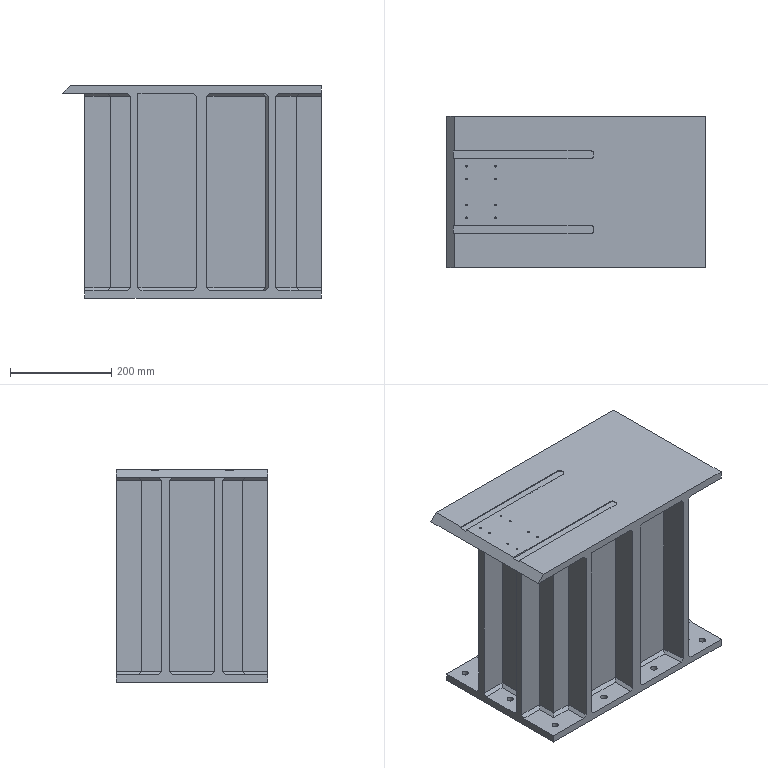Part | Creo | features CUT 7, CURVE 6, DATUM PLANE 3, MOVE 3, CHAMFER 2, PROTRUSION 2, COORDINATE SYSTEM 1, ROUND 1 | 1 solid | 174 faces | box 512 x 300 x 421 mm | volume 36405249 mm3 | plane 134 | cylinder 40 | commonest cylinder face diameters 13 x20 3.3 x16 10 x4